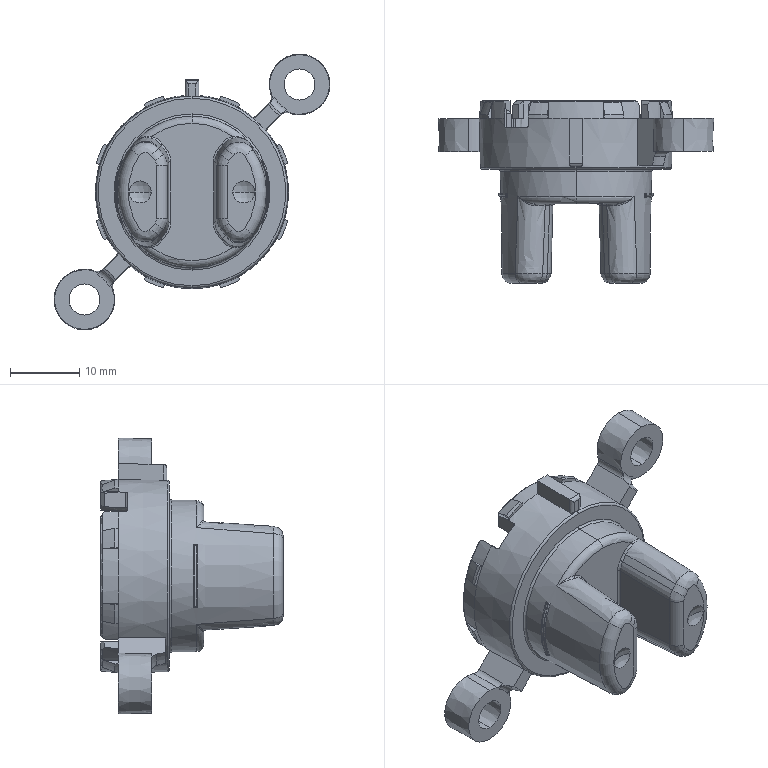Part | STEP file | TBS1007_P12_U_1 | 1 solid | 421 faces | box 39.913 x 26.4 x 39.913 mm | volume 4035 mm3 | plane 164 | cone 94 | spline 82 | cylinder 32 | torus 31 | sphere 18 | commonest cylinder face diameters 0.2 x8 2 x8 1 x7 0.6 x5 3 x2 22.3 x2